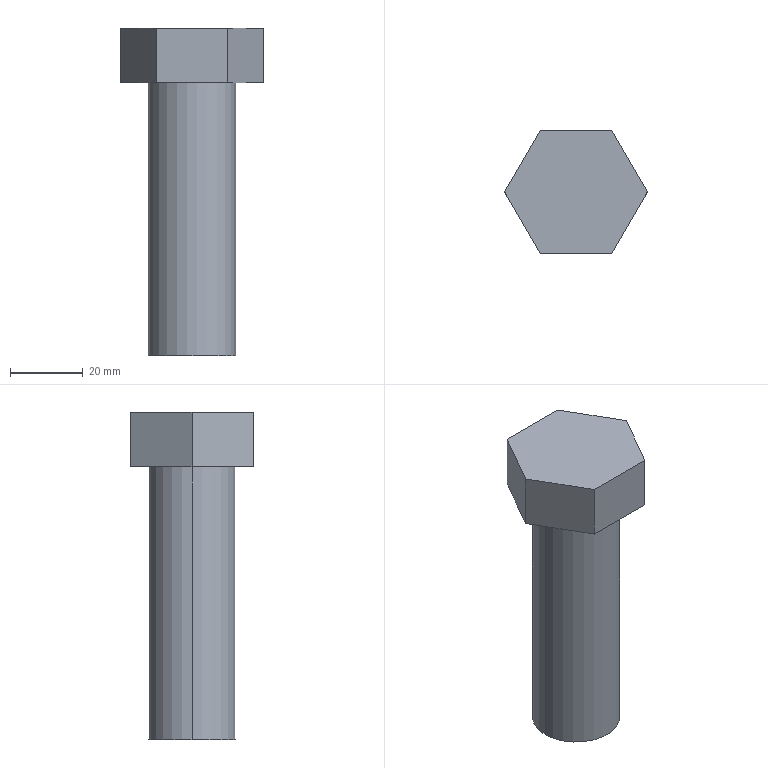Part | STEP file | PN_0027 Punch screw rod | 1 solid | 11 faces | box 39.26 x 34 x 90 mm | volume 48946 mm3 | plane 9 | cylinder 2 | commonest cylinder face diameters 24 x2
STEP:
#1=CARTESIAN_POINT('',(0.,0.,0.));
#2=DIRECTION('',(0.,0.,1.));
#3=DIRECTION('',(1.,0.,0.));
#4=AXIS2_PLACEMENT_3D('',#1,#2,#3);
#5=CARTESIAN_POINT('',(-12.,0.,75.));
#6=VERTEX_POINT('',#5);
#7=CARTESIAN_POINT('',(12.,0.,75.));
#8=VERTEX_POINT('',#7);
#9=CARTESIAN_POINT('',(0.,0.,75.));
#10=DIRECTION('',(0.,0.,-1.));
#11=DIRECTION('',(-1.,0.,0.));
#12=AXIS2_PLACEMENT_3D('',#9,#10,#11);
#13=CIRCLE('',#12,12.);
#14=CARTESIAN_POINT('',(0.,0.,75.));
#15=DIRECTION('',(0.,0.,-1.));
#16=DIRECTION('',(-1.,0.,0.));
#17=AXIS2_PLACEMENT_3D('',#14,#15,#16);
#18=CYLINDRICAL_SURFACE('',#17,12.);
#19=CARTESIAN_POINT('',(0.,0.));
#20=DIRECTION('',(1.,0.));
#21=VECTOR('',#20,1.);
#22=LINE('',#19,#21);
#23=(GEOMETRIC_REPRESENTATION_CONTEXT(2)PARAMETRIC_REPRESENTATION_CONTEXT()REPRESENTATION_CONTEXT('',''));
#24=DEFINITIONAL_REPRESENTATION('',(#22),#23);
#25=PCURVE('',#18,#24);
#26=CARTESIAN_POINT('',(0.,0.,75.));
#27=DIRECTION('',(0.,0.,1.));
#28=DIRECTION('',(1.,0.,0.));
#29=AXIS2_PLACEMENT_3D('',#26,#27,#28);
#30=PLANE('',#29);
#31=CARTESIAN_POINT('',(-12.,0.));
#32=CARTESIAN_POINT('',(-12.,20.785));
#33=CARTESIAN_POINT('',(6.,10.392));
#34=CARTESIAN_POINT('',(24.,0.));
#35=CARTESIAN_POINT('',(6.,-10.392));
#36=CARTESIAN_POINT('',(-12.,-20.785));
#37=CARTESIAN_POINT('',(-12.,0.));
#38=(BOUNDED_CURVE()B_SPLINE_CURVE(2,(#31,#32,#33,#34,#35,#36,#37),.UNSPECIFIED.,.T.,.F.)B_SPLINE_CURVE_WITH_KNOTS((1,2,2,2,2,1),(-2.094,0.,2.094,4.189,6.283,8.378),.UNSPECIFIED.)CURVE()GEOMETRIC_REPRESENTATION_ITEM()RATIONAL_B_SPLINE_CURVE((1.,0.5,1.,0.5,1.,0.5,1.))REPRESENTATION_ITEM(''));
#39=(GEOMETRIC_REPRESENTATION_CONTEXT(2)PARAMETRIC_REPRESENTATION_CONTEXT()REPRESENTATION_CONTEXT('',''));
#40=DEFINITIONAL_REPRESENTATION('',(#38),#39);
#41=PCURVE('',#30,#40);
#42=SURFACE_CURVE('',#13,(#25,#41),.PCURVE_S1.);
#43=EDGE_CURVE('',#6,#8,#42,.T.);
#44=ORIENTED_EDGE('',*,*,#43,.T.);
#45=CARTESIAN_POINT('',(12.,0.,0.));
#46=VERTEX_POINT('',#45);
#47=CARTESIAN_POINT('',(12.,0.,75.));
#48=DIRECTION('',(0.,0.,-1.));
#49=VECTOR('',#48,1.);
#50=LINE('',#47,#49);
#51=CARTESIAN_POINT('',(3.142,0.));
#52=DIRECTION('',(0.,1.));
#53=VECTOR('',#52,1.);
#54=LINE('',#51,#53);
#55=(GEOMETRIC_REPRESENTATION_CONTEXT(2)PARAMETRIC_REPRESENTATION_CONTEXT()REPRESENTATION_CONTEXT('',''));
#56=DEFINITIONAL_REPRESENTATION('',(#54),#55);
#57=PCURVE('',#18,#56);
#58=CARTESIAN_POINT('',(0.,0.,75.));
#59=DIRECTION('',(0.,0.,-1.));
#60=DIRECTION('',(-1.,0.,0.));
#61=AXIS2_PLACEMENT_3D('',#58,#59,#60);
#62=CYLINDRICAL_SURFACE('',#61,12.);
#63=CARTESIAN_POINT('',(3.142,0.));
#64=DIRECTION('',(0.,1.));
#65=VECTOR('',#64,1.);
#66=LINE('',#63,#65);
#67=(GEOMETRIC_REPRESENTATION_CONTEXT(2)PARAMETRIC_REPRESENTATION_CONTEXT()REPRESENTATION_CONTEXT('',''));
#68=DEFINITIONAL_REPRESENTATION('',(#66),#67);
#69=PCURVE('',#62,#68);
#70=SURFACE_CURVE('',#50,(#57,#69),.PCURVE_S1.);
#71=EDGE_CURVE('',#8,#46,#70,.T.);
#72=ORIENTED_EDGE('',*,*,#71,.T.);
#73=CARTESIAN_POINT('',(-12.,0.,0.));
#74=VERTEX_POINT('',#73);
#75=CARTESIAN_POINT('',(0.,0.,0.));
#76=DIRECTION('',(0.,0.,1.));
#77=DIRECTION('',(-1.,0.,0.));
#78=AXIS2_PLACEMENT_3D('',#75,#76,#77);
#79=CIRCLE('',#78,12.);
#80=CARTESIAN_POINT('',(6.283,75.));
#81=DIRECTION('',(-1.,0.));
#82=VECTOR('',#81,1.);
#83=LINE('',#80,#82);
#84=(GEOMETRIC_REPRESENTATION_CONTEXT(2)PARAMETRIC_REPRESENTATION_CONTEXT()REPRESENTATION_CONTEXT('',''));
#85=DEFINITIONAL_REPRESENTATION('',(#83),#84);
#86=PCURVE('',#18,#85);
#87=CARTESIAN_POINT('',(0.,0.,0.));
#88=DIRECTION('',(0.,0.,1.));
#89=DIRECTION('',(1.,0.,0.));
#90=AXIS2_PLACEMENT_3D('',#87,#88,#89);
#91=PLANE('',#90);
#92=CARTESIAN_POINT('',(0.,0.));
#93=DIRECTION('',(-1.,0.));
#94=AXIS2_PLACEMENT_2D('',#92,#93);
#95=CIRCLE('',#94,12.);
#96=(GEOMETRIC_REPRESENTATION_CONTEXT(2)PARAMETRIC_REPRESENTATION_CONTEXT()REPRESENTATION_CONTEXT('',''));
#97=DEFINITIONAL_REPRESENTATION('',(#95),#96);
#98=PCURVE('',#91,#97);
#99=SURFACE_CURVE('',#79,(#86,#98),.PCURVE_S1.);
#100=EDGE_CURVE('',#46,#74,#99,.T.);
#101=ORIENTED_EDGE('',*,*,#100,.T.);
#102=CARTESIAN_POINT('',(-12.,0.,75.));
#103=DIRECTION('',(0.,0.,-1.));
#104=VECTOR('',#103,1.);
#105=LINE('',#102,#104);
#106=CARTESIAN_POINT('',(0.,0.));
#107=DIRECTION('',(0.,1.));
#108=VECTOR('',#107,1.);
#109=LINE('',#106,#108);
#110=(GEOMETRIC_REPRESENTATION_CONTEXT(2)PARAMETRIC_REPRESENTATION_CONTEXT()REPRESENTATION_CONTEXT('',''));
#111=DEFINITIONAL_REPRESENTATION('',(#109),#110);
#112=PCURVE('',#18,#111);
#113=CARTESIAN_POINT('',(6.283,0.));
#114=DIRECTION('',(0.,1.));
#115=VECTOR('',#114,1.);
#116=LINE('',#113,#115);
#117=(GEOMETRIC_REPRESENTATION_CONTEXT(2)PARAMETRIC_REPRESENTATION_CONTEXT()REPRESENTATION_CONTEXT('',''));
#118=DEFINITIONAL_REPRESENTATION('',(#116),#117);
#119=PCURVE('',#62,#118);
#120=SURFACE_CURVE('',#105,(#112,#119),.PCURVE_S1.);
#121=EDGE_CURVE('',#6,#74,#120,.T.);
#122=ORIENTED_EDGE('',*,*,#121,.F.);
#123=EDGE_LOOP('',(#44,#72,#101,#122));
#124=FACE_BOUND('',#123,.T.);
#125=ADVANCED_FACE('',(#124),#18,.T.);
#126=ORIENTED_EDGE('',*,*,#71,.F.);
#127=CARTESIAN_POINT('',(0.,0.,75.));
#128=DIRECTION('',(0.,0.,-1.));
#129=DIRECTION('',(-1.,0.,0.));
#130=AXIS2_PLACEMENT_3D('',#127,#128,#129);
#131=CIRCLE('',#130,12.);
#132=CARTESIAN_POINT('',(0.,0.));
#133=DIRECTION('',(1.,0.));
#134=VECTOR('',#133,1.);
#135=LINE('',#132,#134);
#136=(GEOMETRIC_REPRESENTATION_CONTEXT(2)PARAMETRIC_REPRESENTATION_CONTEXT()REPRESENTATION_CONTEXT('',''));
#137=DEFINITIONAL_REPRESENTATION('',(#135),#136);
#138=PCURVE('',#62,#137);
#139=CARTESIAN_POINT('',(-12.,0.));
#140=CARTESIAN_POINT('',(-12.,20.785));
#141=CARTESIAN_POINT('',(6.,10.392));
#142=CARTESIAN_POINT('',(24.,0.));
#143=CARTESIAN_POINT('',(6.,-10.392));
#144=CARTESIAN_POINT('',(-12.,-20.785));
#145=CARTESIAN_POINT('',(-12.,0.));
#146=(BOUNDED_CURVE()B_SPLINE_CURVE(2,(#139,#140,#141,#142,#143,#144,#145),.UNSPECIFIED.,.T.,.F.)B_SPLINE_CURVE_WITH_KNOTS((1,2,2,2,2,1),(-2.094,0.,2.094,4.189,6.283,8.378),.UNSPECIFIED.)CURVE()GEOMETRIC_REPRESENTATION_ITEM()RATIONAL_B_SPLINE_CURVE((1.,0.5,1.,0.5,1.,0.5,1.))REPRESENTATION_ITEM(''));
#147=(GEOMETRIC_REPRESENTATION_CONTEXT(2)PARAMETRIC_REPRESENTATION_CONTEXT()REPRESENTATION_CONTEXT('',''));
#148=DEFINITIONAL_REPRESENTATION('',(#146),#147);
#149=PCURVE('',#30,#148);
#150=SURFACE_CURVE('',#131,(#138,#149),.PCURVE_S1.);
#151=EDGE_CURVE('',#8,#6,#150,.T.);
#152=ORIENTED_EDGE('',*,*,#151,.T.);
#153=ORIENTED_EDGE('',*,*,#121,.T.);
#154=CARTESIAN_POINT('',(0.,0.,0.));
#155=DIRECTION('',(0.,0.,1.));
#156=DIRECTION('',(-1.,0.,0.));
#157=AXIS2_PLACEMENT_3D('',#154,#155,#156);
#158=CIRCLE('',#157,12.);
#159=CARTESIAN_POINT('',(6.283,75.));
#160=DIRECTION('',(-1.,0.));
#161=VECTOR('',#160,1.);
#162=LINE('',#159,#161);
#163=(GEOMETRIC_REPRESENTATION_CONTEXT(2)PARAMETRIC_REPRESENTATION_CONTEXT()REPRESENTATION_CONTEXT('',''));
#164=DEFINITIONAL_REPRESENTATION('',(#162),#163);
#165=PCURVE('',#62,#164);
#166=CARTESIAN_POINT('',(0.,0.));
#167=DIRECTION('',(-1.,0.));
#168=AXIS2_PLACEMENT_2D('',#166,#167);
#169=CIRCLE('',#168,12.);
#170=(GEOMETRIC_REPRESENTATION_CONTEXT(2)PARAMETRIC_REPRESENTATION_CONTEXT()REPRESENTATION_CONTEXT('',''));
#171=DEFINITIONAL_REPRESENTATION('',(#169),#170);
#172=PCURVE('',#91,#171);
#173=SURFACE_CURVE('',#158,(#165,#172),.PCURVE_S1.);
#174=EDGE_CURVE('',#74,#46,#173,.T.);
#175=ORIENTED_EDGE('',*,*,#174,.T.);
#176=EDGE_LOOP('',(#126,#152,#153,#175));
#177=FACE_BOUND('',#176,.T.);
#178=ADVANCED_FACE('',(#177),#62,.T.);
#179=ORIENTED_EDGE('',*,*,#174,.F.);
#180=ORIENTED_EDGE('',*,*,#100,.F.);
#181=EDGE_LOOP('',(#179,#180));
#182=FACE_BOUND('',#181,.T.);
#183=ADVANCED_FACE('',(#182),#91,.F.);
#184=ORIENTED_EDGE('',*,*,#43,.F.);
#185=ORIENTED_EDGE('',*,*,#151,.F.);
#186=EDGE_LOOP('',(#184,#185));
#187=FACE_BOUND('',#186,.T.);
#188=CARTESIAN_POINT('',(-9.815,-17.,75.));
#189=VERTEX_POINT('',#188);
#190=CARTESIAN_POINT('',(9.815,-17.,75.));
#191=VERTEX_POINT('',#190);
#192=CARTESIAN_POINT('',(0.,-17.,75.));
#193=DIRECTION('',(1.,0.,0.));
#194=VECTOR('',#193,1.);
#195=LINE('',#192,#194);
#196=CARTESIAN_POINT('',(0.,-17.));
#197=DIRECTION('',(1.,0.));
#198=VECTOR('',#197,1.);
#199=LINE('',#196,#198);
#200=(GEOMETRIC_REPRESENTATION_CONTEXT(2)PARAMETRIC_REPRESENTATION_CONTEXT()REPRESENTATION_CONTEXT('',''));
#201=DEFINITIONAL_REPRESENTATION('',(#199),#200);
#202=PCURVE('',#30,#201);
#203=CARTESIAN_POINT('',(-9.815,-17.,90.));
#204=DIRECTION('',(0.,1.,0.));
#205=DIRECTION('',(-1.,0.,0.));
#206=AXIS2_PLACEMENT_3D('',#203,#204,#205);
#207=PLANE('',#206);
#208=CARTESIAN_POINT('',(-9.815,-15.));
#209=DIRECTION('',(-1.,0.));
#210=VECTOR('',#209,1.);
#211=LINE('',#208,#210);
#212=(GEOMETRIC_REPRESENTATION_CONTEXT(2)PARAMETRIC_REPRESENTATION_CONTEXT()REPRESENTATION_CONTEXT('',''));
#213=DEFINITIONAL_REPRESENTATION('',(#211),#212);
#214=PCURVE('',#207,#213);
#215=SURFACE_CURVE('',#195,(#202,#214),.PCURVE_S1.);
#216=EDGE_CURVE('',#189,#191,#215,.T.);
#217=ORIENTED_EDGE('',*,*,#216,.F.);
#218=CARTESIAN_POINT('',(-19.63,0.,75.));
#219=VERTEX_POINT('',#218);
#220=CARTESIAN_POINT('',(-19.63,0.,75.));
#221=DIRECTION('',(0.5,-0.866,0.));
#222=VECTOR('',#221,1.);
#223=LINE('',#220,#222);
#224=CARTESIAN_POINT('',(-19.63,0.));
#225=DIRECTION('',(0.5,-0.866));
#226=VECTOR('',#225,1.);
#227=LINE('',#224,#226);
#228=(GEOMETRIC_REPRESENTATION_CONTEXT(2)PARAMETRIC_REPRESENTATION_CONTEXT()REPRESENTATION_CONTEXT('',''));
#229=DEFINITIONAL_REPRESENTATION('',(#227),#228);
#230=PCURVE('',#30,#229);
#231=CARTESIAN_POINT('',(-19.63,0.,90.));
#232=DIRECTION('',(0.866,0.5,0.));
#233=DIRECTION('',(-0.5,0.866,0.));
#234=AXIS2_PLACEMENT_3D('',#231,#232,#233);
#235=PLANE('',#234);
#236=CARTESIAN_POINT('',(0.,-15.));
#237=DIRECTION('',(-1.,0.));
#238=VECTOR('',#237,1.);
#239=LINE('',#236,#238);
#240=(GEOMETRIC_REPRESENTATION_CONTEXT(2)PARAMETRIC_REPRESENTATION_CONTEXT()REPRESENTATION_CONTEXT('',''));
#241=DEFINITIONAL_REPRESENTATION('',(#239),#240);
#242=PCURVE('',#235,#241);
#243=SURFACE_CURVE('',#223,(#230,#242),.PCURVE_S1.);
#244=EDGE_CURVE('',#219,#189,#243,.T.);
#245=ORIENTED_EDGE('',*,*,#244,.F.);
#246=CARTESIAN_POINT('',(-9.815,17.,75.));
#247=VERTEX_POINT('',#246);
#248=CARTESIAN_POINT('',(-9.815,17.,75.));
#249=DIRECTION('',(-0.5,-0.866,0.));
#250=VECTOR('',#249,1.);
#251=LINE('',#248,#250);
#252=CARTESIAN_POINT('',(-9.815,17.));
#253=DIRECTION('',(-0.5,-0.866));
#254=VECTOR('',#253,1.);
#255=LINE('',#252,#254);
#256=(GEOMETRIC_REPRESENTATION_CONTEXT(2)PARAMETRIC_REPRESENTATION_CONTEXT()REPRESENTATION_CONTEXT('',''));
#257=DEFINITIONAL_REPRESENTATION('',(#255),#256);
#258=PCURVE('',#30,#257);
#259=CARTESIAN_POINT('',(-9.815,17.,90.));
#260=DIRECTION('',(0.866,-0.5,0.));
#261=DIRECTION('',(0.5,0.866,0.));
#262=AXIS2_PLACEMENT_3D('',#259,#260,#261);
#263=PLANE('',#262);
#264=CARTESIAN_POINT('',(0.,-15.));
#265=DIRECTION('',(-1.,0.));
#266=VECTOR('',#265,1.);
#267=LINE('',#264,#266);
#268=(GEOMETRIC_REPRESENTATION_CONTEXT(2)PARAMETRIC_REPRESENTATION_CONTEXT()REPRESENTATION_CONTEXT('',''));
#269=DEFINITIONAL_REPRESENTATION('',(#267),#268);
#270=PCURVE('',#263,#269);
#271=SURFACE_CURVE('',#251,(#258,#270),.PCURVE_S1.);
#272=EDGE_CURVE('',#247,#219,#271,.T.);
#273=ORIENTED_EDGE('',*,*,#272,.F.);
#274=CARTESIAN_POINT('',(9.815,17.,75.));
#275=VERTEX_POINT('',#274);
#276=CARTESIAN_POINT('',(0.,17.,75.));
#277=DIRECTION('',(-1.,0.,0.));
#278=VECTOR('',#277,1.);
#279=LINE('',#276,#278);
#280=CARTESIAN_POINT('',(0.,17.));
#281=DIRECTION('',(-1.,0.));
#282=VECTOR('',#281,1.);
#283=LINE('',#280,#282);
#284=(GEOMETRIC_REPRESENTATION_CONTEXT(2)PARAMETRIC_REPRESENTATION_CONTEXT()REPRESENTATION_CONTEXT('',''));
#285=DEFINITIONAL_REPRESENTATION('',(#283),#284);
#286=PCURVE('',#30,#285);
#287=CARTESIAN_POINT('',(9.815,17.,90.));
#288=DIRECTION('',(0.,-1.,0.));
#289=DIRECTION('',(1.,0.,0.));
#290=AXIS2_PLACEMENT_3D('',#287,#288,#289);
#291=PLANE('',#290);
#292=CARTESIAN_POINT('',(-9.815,-15.));
#293=DIRECTION('',(-1.,0.));
#294=VECTOR('',#293,1.);
#295=LINE('',#292,#294);
#296=(GEOMETRIC_REPRESENTATION_CONTEXT(2)PARAMETRIC_REPRESENTATION_CONTEXT()REPRESENTATION_CONTEXT('',''));
#297=DEFINITIONAL_REPRESENTATION('',(#295),#296);
#298=PCURVE('',#291,#297);
#299=SURFACE_CURVE('',#279,(#286,#298),.PCURVE_S1.);
#300=EDGE_CURVE('',#275,#247,#299,.T.);
#301=ORIENTED_EDGE('',*,*,#300,.F.);
#302=CARTESIAN_POINT('',(19.63,0.,75.));
#303=VERTEX_POINT('',#302);
#304=CARTESIAN_POINT('',(19.63,0.,75.));
#305=DIRECTION('',(-0.5,0.866,0.));
#306=VECTOR('',#305,1.);
#307=LINE('',#304,#306);
#308=CARTESIAN_POINT('',(19.63,0.));
#309=DIRECTION('',(-0.5,0.866));
#310=VECTOR('',#309,1.);
#311=LINE('',#308,#310);
#312=(GEOMETRIC_REPRESENTATION_CONTEXT(2)PARAMETRIC_REPRESENTATION_CONTEXT()REPRESENTATION_CONTEXT('',''));
#313=DEFINITIONAL_REPRESENTATION('',(#311),#312);
#314=PCURVE('',#30,#313);
#315=CARTESIAN_POINT('',(19.63,0.,90.));
#316=DIRECTION('',(-0.866,-0.5,0.));
#317=DIRECTION('',(0.5,-0.866,0.));
#318=AXIS2_PLACEMENT_3D('',#315,#316,#317);
#319=PLANE('',#318);
#320=CARTESIAN_POINT('',(0.,-15.));
#321=DIRECTION('',(-1.,0.));
#322=VECTOR('',#321,1.);
#323=LINE('',#320,#322);
#324=(GEOMETRIC_REPRESENTATION_CONTEXT(2)PARAMETRIC_REPRESENTATION_CONTEXT()REPRESENTATION_CONTEXT('',''));
#325=DEFINITIONAL_REPRESENTATION('',(#323),#324);
#326=PCURVE('',#319,#325);
#327=SURFACE_CURVE('',#307,(#314,#326),.PCURVE_S1.);
#328=EDGE_CURVE('',#303,#275,#327,.T.);
#329=ORIENTED_EDGE('',*,*,#328,.F.);
#330=CARTESIAN_POINT('',(9.815,-17.,75.));
#331=DIRECTION('',(0.5,0.866,0.));
#332=VECTOR('',#331,1.);
#333=LINE('',#330,#332);
#334=CARTESIAN_POINT('',(9.815,-17.));
#335=DIRECTION('',(0.5,0.866));
#336=VECTOR('',#335,1.);
#337=LINE('',#334,#336);
#338=(GEOMETRIC_REPRESENTATION_CONTEXT(2)PARAMETRIC_REPRESENTATION_CONTEXT()REPRESENTATION_CONTEXT('',''));
#339=DEFINITIONAL_REPRESENTATION('',(#337),#338);
#340=PCURVE('',#30,#339);
#341=CARTESIAN_POINT('',(9.815,-17.,90.));
#342=DIRECTION('',(-0.866,0.5,0.));
#343=DIRECTION('',(-0.5,-0.866,0.));
#344=AXIS2_PLACEMENT_3D('',#341,#342,#343);
#345=PLANE('',#344);
#346=CARTESIAN_POINT('',(0.,-15.));
#347=DIRECTION('',(-1.,0.));
#348=VECTOR('',#347,1.);
#349=LINE('',#346,#348);
#350=(GEOMETRIC_REPRESENTATION_CONTEXT(2)PARAMETRIC_REPRESENTATION_CONTEXT()REPRESENTATION_CONTEXT('',''));
#351=DEFINITIONAL_REPRESENTATION('',(#349),#350);
#352=PCURVE('',#345,#351);
#353=SURFACE_CURVE('',#333,(#340,#352),.PCURVE_S1.);
#354=EDGE_CURVE('',#191,#303,#353,.T.);
#355=ORIENTED_EDGE('',*,*,#354,.F.);
#356=EDGE_LOOP('',(#217,#245,#273,#301,#329,#355));
#357=FACE_BOUND('',#356,.T.);
#358=ADVANCED_FACE('',(#187,#357),#30,.F.);
#359=CARTESIAN_POINT('',(19.63,0.,90.));
#360=VERTEX_POINT('',#359);
#361=CARTESIAN_POINT('',(19.63,0.,90.));
#362=DIRECTION('',(0.,0.,-1.));
#363=VECTOR('',#362,1.);
#364=LINE('',#361,#363);
#365=CARTESIAN_POINT('',(-19.63,0.));
#366=DIRECTION('',(0.,-1.));
#367=VECTOR('',#366,1.);
#368=LINE('',#365,#367);
#369=(GEOMETRIC_REPRESENTATION_CONTEXT(2)PARAMETRIC_REPRESENTATION_CONTEXT()REPRESENTATION_CONTEXT('',''));
#370=DEFINITIONAL_REPRESENTATION('',(#368),#369);
#371=PCURVE('',#345,#370);
#372=CARTESIAN_POINT('',(0.,0.));
#373=DIRECTION('',(0.,-1.));
#374=VECTOR('',#373,1.);
#375=LINE('',#372,#374);
#376=(GEOMETRIC_REPRESENTATION_CONTEXT(2)PARAMETRIC_REPRESENTATION_CONTEXT()REPRESENTATION_CONTEXT('',''));
#377=DEFINITIONAL_REPRESENTATION('',(#375),#376);
#378=PCURVE('',#319,#377);
#379=SURFACE_CURVE('',#364,(#371,#378),.PCURVE_S1.);
#380=EDGE_CURVE('',#360,#303,#379,.T.);
#381=ORIENTED_EDGE('',*,*,#380,.F.);
#382=CARTESIAN_POINT('',(9.815,-17.,90.));
#383=VERTEX_POINT('',#382);
#384=CARTESIAN_POINT('',(9.815,-17.,90.));
#385=DIRECTION('',(0.5,0.866,0.));
#386=VECTOR('',#385,1.);
#387=LINE('',#384,#386);
#388=CARTESIAN_POINT('',(0.,0.));
#389=DIRECTION('',(-1.,0.));
#390=VECTOR('',#389,1.);
#391=LINE('',#388,#390);
#392=(GEOMETRIC_REPRESENTATION_CONTEXT(2)PARAMETRIC_REPRESENTATION_CONTEXT()REPRESENTATION_CONTEXT('',''));
#393=DEFINITIONAL_REPRESENTATION('',(#391),#392);
#394=PCURVE('',#345,#393);
#395=CARTESIAN_POINT('',(0.,0.,90.));
#396=DIRECTION('',(0.,0.,1.));
#397=DIRECTION('',(1.,0.,0.));
#398=AXIS2_PLACEMENT_3D('',#395,#396,#397);
#399=PLANE('',#398);
#400=CARTESIAN_POINT('',(9.815,-17.));
#401=DIRECTION('',(0.5,0.866));
#402=VECTOR('',#401,1.);
#403=LINE('',#400,#402);
#404=(GEOMETRIC_REPRESENTATION_CONTEXT(2)PARAMETRIC_REPRESENTATION_CONTEXT()REPRESENTATION_CONTEXT('',''));
#405=DEFINITIONAL_REPRESENTATION('',(#403),#404);
#406=PCURVE('',#399,#405);
#407=SURFACE_CURVE('',#387,(#394,#406),.PCURVE_S1.);
#408=EDGE_CURVE('',#383,#360,#407,.T.);
#409=ORIENTED_EDGE('',*,*,#408,.F.);
#410=CARTESIAN_POINT('',(9.815,-17.,90.));
#411=DIRECTION('',(0.,0.,1.));
#412=VECTOR('',#411,1.);
#413=LINE('',#410,#412);
#414=CARTESIAN_POINT('',(0.,0.));
#415=DIRECTION('',(0.,1.));
#416=VECTOR('',#415,1.);
#417=LINE('',#414,#416);
#418=(GEOMETRIC_REPRESENTATION_CONTEXT(2)PARAMETRIC_REPRESENTATION_CONTEXT()REPRESENTATION_CONTEXT('',''));
#419=DEFINITIONAL_REPRESENTATION('',(#417),#418);
#420=PCURVE('',#345,#419);
#421=CARTESIAN_POINT('',(-19.63,0.));
#422=DIRECTION('',(0.,1.));
#423=VECTOR('',#422,1.);
#424=LINE('',#421,#423);
#425=(GEOMETRIC_REPRESENTATION_CONTEXT(2)PARAMETRIC_REPRESENTATION_CONTEXT()REPRESENTATION_CONTEXT('',''));
#426=DEFINITIONAL_REPRESENTATION('',(#424),#425);
#427=PCURVE('',#207,#426);
#428=SURFACE_CURVE('',#413,(#420,#427),.PCURVE_S1.);
#429=EDGE_CURVE('',#191,#383,#428,.T.);
#430=ORIENTED_EDGE('',*,*,#429,.F.);
#431=ORIENTED_EDGE('',*,*,#354,.T.);
#432=EDGE_LOOP('',(#381,#409,#430,#431));
#433=FACE_BOUND('',#432,.T.);
#434=ADVANCED_FACE('',(#433),#345,.F.);
#435=ORIENTED_EDGE('',*,*,#429,.T.);
#436=CARTESIAN_POINT('',(-9.815,-17.,90.));
#437=VERTEX_POINT('',#436);
#438=CARTESIAN_POINT('',(-9.815,-17.,90.));
#439=DIRECTION('',(1.,0.,0.));
#440=VECTOR('',#439,1.);
#441=LINE('',#438,#440);
#442=CARTESIAN_POINT('',(0.,0.));
#443=DIRECTION('',(-1.,0.));
#444=VECTOR('',#443,1.);
#445=LINE('',#442,#444);
#446=(GEOMETRIC_REPRESENTATION_CONTEXT(2)PARAMETRIC_REPRESENTATION_CONTEXT()REPRESENTATION_CONTEXT('',''));
#447=DEFINITIONAL_REPRESENTATION('',(#445),#446);
#448=PCURVE('',#207,#447);
#449=CARTESIAN_POINT('',(-9.815,-17.));
#450=DIRECTION('',(1.,0.));
#451=VECTOR('',#450,1.);
#452=LINE('',#449,#451);
#453=(GEOMETRIC_REPRESENTATION_CONTEXT(2)PARAMETRIC_REPRESENTATION_CONTEXT()REPRESENTATION_CONTEXT('',''));
#454=DEFINITIONAL_REPRESENTATION('',(#452),#453);
#455=PCURVE('',#399,#454);
#456=SURFACE_CURVE('',#441,(#448,#455),.PCURVE_S1.);
#457=EDGE_CURVE('',#437,#383,#456,.T.);
#458=ORIENTED_EDGE('',*,*,#457,.F.);
#459=CARTESIAN_POINT('',(-9.815,-17.,90.));
#460=DIRECTION('',(0.,0.,1.));
#461=VECTOR('',#460,1.);
#462=LINE('',#459,#461);
#463=CARTESIAN_POINT('',(0.,0.));
#464=DIRECTION('',(0.,1.));
#465=VECTOR('',#464,1.);
#466=LINE('',#463,#465);
#467=(GEOMETRIC_REPRESENTATION_CONTEXT(2)PARAMETRIC_REPRESENTATION_CONTEXT()REPRESENTATION_CONTEXT('',''));
#468=DEFINITIONAL_REPRESENTATION('',(#466),#467);
#469=PCURVE('',#207,#468);
#470=CARTESIAN_POINT('',(-19.63,0.));
#471=DIRECTION('',(0.,1.));
#472=VECTOR('',#471,1.);
#473=LINE('',#470,#472);
#474=(GEOMETRIC_REPRESENTATION_CONTEXT(2)PARAMETRIC_REPRESENTATION_CONTEXT()REPRESENTATION_CONTEXT('',''));
#475=DEFINITIONAL_REPRESENTATION('',(#473),#474);
#476=PCURVE('',#235,#475);
#477=SURFACE_CURVE('',#462,(#469,#476),.PCURVE_S1.);
#478=EDGE_CURVE('',#189,#437,#477,.T.);
#479=ORIENTED_EDGE('',*,*,#478,.F.);
#480=ORIENTED_EDGE('',*,*,#216,.T.);
#481=EDGE_LOOP('',(#435,#458,#479,#480));
#482=FACE_BOUND('',#481,.T.);
#483=ADVANCED_FACE('',(#482),#207,.F.);
#484=ORIENTED_EDGE('',*,*,#478,.T.);
#485=CARTESIAN_POINT('',(-19.63,0.,90.));
#486=VERTEX_POINT('',#485);
#487=CARTESIAN_POINT('',(-19.63,0.,90.));
#488=DIRECTION('',(0.5,-0.866,0.));
#489=VECTOR('',#488,1.);
#490=LINE('',#487,#489);
#491=CARTESIAN_POINT('',(0.,0.));
#492=DIRECTION('',(-1.,0.));
#493=VECTOR('',#492,1.);
#494=LINE('',#491,#493);
#495=(GEOMETRIC_REPRESENTATION_CONTEXT(2)PARAMETRIC_REPRESENTATION_CONTEXT()REPRESENTATION_CONTEXT('',''));
#496=DEFINITIONAL_REPRESENTATION('',(#494),#495);
#497=PCURVE('',#235,#496);
#498=CARTESIAN_POINT('',(-19.63,0.));
#499=DIRECTION('',(0.5,-0.866));
#500=VECTOR('',#499,1.);
#501=LINE('',#498,#500);
#502=(GEOMETRIC_REPRESENTATION_CONTEXT(2)PARAMETRIC_REPRESENTATION_CONTEXT()REPRESENTATION_CONTEXT('',''));
#503=DEFINITIONAL_REPRESENTATION('',(#501),#502);
#504=PCURVE('',#399,#503);
#505=SURFACE_CURVE('',#490,(#497,#504),.PCURVE_S1.);
#506=EDGE_CURVE('',#486,#437,#505,.T.);
#507=ORIENTED_EDGE('',*,*,#506,.F.);
#508=CARTESIAN_POINT('',(-19.63,0.,90.));
#509=DIRECTION('',(0.,0.,1.));
#510=VECTOR('',#509,1.);
#511=LINE('',#508,#510);
#512=CARTESIAN_POINT('',(0.,0.));
#513=DIRECTION('',(0.,1.));
#514=VECTOR('',#513,1.);
#515=LINE('',#512,#514);
#516=(GEOMETRIC_REPRESENTATION_CONTEXT(2)PARAMETRIC_REPRESENTATION_CONTEXT()REPRESENTATION_CONTEXT('',''));
#517=DEFINITIONAL_REPRESENTATION('',(#515),#516);
#518=PCURVE('',#235,#517);
#519=CARTESIAN_POINT('',(-19.63,0.));
#520=DIRECTION('',(0.,1.));
#521=VECTOR('',#520,1.);
#522=LINE('',#519,#521);
#523=(GEOMETRIC_REPRESENTATION_CONTEXT(2)PARAMETRIC_REPRESENTATION_CONTEXT()REPRESENTATION_CONTEXT('',''));
#524=DEFINITIONAL_REPRESENTATION('',(#522),#523);
#525=PCURVE('',#263,#524);
#526=SURFACE_CURVE('',#511,(#518,#525),.PCURVE_S1.);
#527=EDGE_CURVE('',#219,#486,#526,.T.);
#528=ORIENTED_EDGE('',*,*,#527,.F.);
#529=ORIENTED_EDGE('',*,*,#244,.T.);
#530=EDGE_LOOP('',(#484,#507,#528,#529));
#531=FACE_BOUND('',#530,.T.);
#532=ADVANCED_FACE('',(#531),#235,.F.);
#533=ORIENTED_EDGE('',*,*,#527,.T.);
#534=CARTESIAN_POINT('',(-9.815,17.,90.));
#535=VERTEX_POINT('',#534);
#536=CARTESIAN_POINT('',(-9.815,17.,90.));
#537=DIRECTION('',(-0.5,-0.866,0.));
#538=VECTOR('',#537,1.);
#539=LINE('',#536,#538);
#540=CARTESIAN_POINT('',(0.,0.));
#541=DIRECTION('',(-1.,0.));
#542=VECTOR('',#541,1.);
#543=LINE('',#540,#542);
#544=(GEOMETRIC_REPRESENTATION_CONTEXT(2)PARAMETRIC_REPRESENTATION_CONTEXT()REPRESENTATION_CONTEXT('',''));
#545=DEFINITIONAL_REPRESENTATION('',(#543),#544);
#546=PCURVE('',#263,#545);
#547=CARTESIAN_POINT('',(-9.815,17.));
#548=DIRECTION('',(-0.5,-0.866));
#549=VECTOR('',#548,1.);
#550=LINE('',#547,#549);
#551=(GEOMETRIC_REPRESENTATION_CONTEXT(2)PARAMETRIC_REPRESENTATION_CONTEXT()REPRESENTATION_CONTEXT('',''));
#552=DEFINITIONAL_REPRESENTATION('',(#550),#551);
#553=PCURVE('',#399,#552);
#554=SURFACE_CURVE('',#539,(#546,#553),.PCURVE_S1.);
#555=EDGE_CURVE('',#535,#486,#554,.T.);
#556=ORIENTED_EDGE('',*,*,#555,.F.);
#557=CARTESIAN_POINT('',(-9.815,17.,90.));
#558=DIRECTION('',(0.,0.,1.));
#559=VECTOR('',#558,1.);
#560=LINE('',#557,#559);
#561=CARTESIAN_POINT('',(0.,0.));
#562=DIRECTION('',(0.,1.));
#563=VECTOR('',#562,1.);
#564=LINE('',#561,#563);
#565=(GEOMETRIC_REPRESENTATION_CONTEXT(2)PARAMETRIC_REPRESENTATION_CONTEXT()REPRESENTATION_CONTEXT('',''));
#566=DEFINITIONAL_REPRESENTATION('',(#564),#565);
#567=PCURVE('',#263,#566);
#568=CARTESIAN_POINT('',(-19.63,0.));
#569=DIRECTION('',(0.,1.));
#570=VECTOR('',#569,1.);
#571=LINE('',#568,#570);
#572=(GEOMETRIC_REPRESENTATION_CONTEXT(2)PARAMETRIC_REPRESENTATION_CONTEXT()REPRESENTATION_CONTEXT('',''));
#573=DEFINITIONAL_REPRESENTATION('',(#571),#572);
#574=PCURVE('',#291,#573);
#575=SURFACE_CURVE('',#560,(#567,#574),.PCURVE_S1.);
#576=EDGE_CURVE('',#247,#535,#575,.T.);
#577=ORIENTED_EDGE('',*,*,#576,.F.);
#578=ORIENTED_EDGE('',*,*,#272,.T.);
#579=EDGE_LOOP('',(#533,#556,#577,#578));
#580=FACE_BOUND('',#579,.T.);
#581=ADVANCED_FACE('',(#580),#263,.F.);
#582=ORIENTED_EDGE('',*,*,#576,.T.);
#583=CARTESIAN_POINT('',(9.815,17.,90.));
#584=VERTEX_POINT('',#583);
#585=CARTESIAN_POINT('',(9.815,17.,90.));
#586=DIRECTION('',(-1.,0.,0.));
#587=VECTOR('',#586,1.);
#588=LINE('',#585,#587);
#589=CARTESIAN_POINT('',(0.,0.));
#590=DIRECTION('',(-1.,0.));
#591=VECTOR('',#590,1.);
#592=LINE('',#589,#591);
#593=(GEOMETRIC_REPRESENTATION_CONTEXT(2)PARAMETRIC_REPRESENTATION_CONTEXT()REPRESENTATION_CONTEXT('',''));
#594=DEFINITIONAL_REPRESENTATION('',(#592),#593);
#595=PCURVE('',#291,#594);
#596=CARTESIAN_POINT('',(9.815,17.));
#597=DIRECTION('',(-1.,0.));
#598=VECTOR('',#597,1.);
#599=LINE('',#596,#598);
#600=(GEOMETRIC_REPRESENTATION_CONTEXT(2)PARAMETRIC_REPRESENTATION_CONTEXT()REPRESENTATION_CONTEXT('',''));
#601=DEFINITIONAL_REPRESENTATION('',(#599),#600);
#602=PCURVE('',#399,#601);
#603=SURFACE_CURVE('',#588,(#595,#602),.PCURVE_S1.);
#604=EDGE_CURVE('',#584,#535,#603,.T.);
#605=ORIENTED_EDGE('',*,*,#604,.F.);
#606=CARTESIAN_POINT('',(9.815,17.,90.));
#607=DIRECTION('',(0.,0.,1.));
#608=VECTOR('',#607,1.);
#609=LINE('',#606,#608);
#610=CARTESIAN_POINT('',(0.,0.));
#611=DIRECTION('',(0.,1.));
#612=VECTOR('',#611,1.);
#613=LINE('',#610,#612);
#614=(GEOMETRIC_REPRESENTATION_CONTEXT(2)PARAMETRIC_REPRESENTATION_CONTEXT()REPRESENTATION_CONTEXT('',''));
#615=DEFINITIONAL_REPRESENTATION('',(#613),#614);
#616=PCURVE('',#291,#615);
#617=CARTESIAN_POINT('',(-19.63,0.));
#618=DIRECTION('',(0.,1.));
#619=VECTOR('',#618,1.);
#620=LINE('',#617,#619);
#621=(GEOMETRIC_REPRESENTATION_CONTEXT(2)PARAMETRIC_REPRESENTATION_CONTEXT()REPRESENTATION_CONTEXT('',''));
#622=DEFINITIONAL_REPRESENTATION('',(#620),#621);
#623=PCURVE('',#319,#622);
#624=SURFACE_CURVE('',#609,(#616,#623),.PCURVE_S1.);
#625=EDGE_CURVE('',#275,#584,#624,.T.);
#626=ORIENTED_EDGE('',*,*,#625,.F.);
#627=ORIENTED_EDGE('',*,*,#300,.T.);
#628=EDGE_LOOP('',(#582,#605,#626,#627));
#629=FACE_BOUND('',#628,.T.);
#630=ADVANCED_FACE('',(#629),#291,.F.);
#631=ORIENTED_EDGE('',*,*,#625,.T.);
#632=CARTESIAN_POINT('',(19.63,0.,90.));
#633=DIRECTION('',(-0.5,0.866,0.));
#634=VECTOR('',#633,1.);
#635=LINE('',#632,#634);
#636=CARTESIAN_POINT('',(0.,0.));
#637=DIRECTION('',(-1.,0.));
#638=VECTOR('',#637,1.);
#639=LINE('',#636,#638);
#640=(GEOMETRIC_REPRESENTATION_CONTEXT(2)PARAMETRIC_REPRESENTATION_CONTEXT()REPRESENTATION_CONTEXT('',''));
#641=DEFINITIONAL_REPRESENTATION('',(#639),#640);
#642=PCURVE('',#319,#641);
#643=CARTESIAN_POINT('',(19.63,0.));
#644=DIRECTION('',(-0.5,0.866));
#645=VECTOR('',#644,1.);
#646=LINE('',#643,#645);
#647=(GEOMETRIC_REPRESENTATION_CONTEXT(2)PARAMETRIC_REPRESENTATION_CONTEXT()REPRESENTATION_CONTEXT('',''));
#648=DEFINITIONAL_REPRESENTATION('',(#646),#647);
#649=PCURVE('',#399,#648);
#650=SURFACE_CURVE('',#635,(#642,#649),.PCURVE_S1.);
#651=EDGE_CURVE('',#360,#584,#650,.T.);
#652=ORIENTED_EDGE('',*,*,#651,.F.);
#653=ORIENTED_EDGE('',*,*,#380,.T.);
#654=ORIENTED_EDGE('',*,*,#328,.T.);
#655=EDGE_LOOP('',(#631,#652,#653,#654));
#656=FACE_BOUND('',#655,.T.);
#657=ADVANCED_FACE('',(#656),#319,.F.);
#658=ORIENTED_EDGE('',*,*,#506,.T.);
#659=ORIENTED_EDGE('',*,*,#457,.T.);
#660=ORIENTED_EDGE('',*,*,#408,.T.);
#661=ORIENTED_EDGE('',*,*,#651,.T.);
#662=ORIENTED_EDGE('',*,*,#604,.T.);
#663=ORIENTED_EDGE('',*,*,#555,.T.);
#664=EDGE_LOOP('',(#658,#659,#660,#661,#662,#663));
#665=FACE_BOUND('',#664,.T.);
#666=ADVANCED_FACE('',(#665),#399,.T.);
#667=CLOSED_SHELL('',(#125,#178,#183,#358,#434,#483,#532,#581,#630,#657,#666));
#668=MANIFOLD_SOLID_BREP('',#667);
#669=(LENGTH_UNIT()NAMED_UNIT(*)SI_UNIT(.MILLI.,.METRE.));
#670=UNCERTAINTY_MEASURE_WITH_UNIT(LENGTH_MEASURE(0.0000001),#669,'','');
#671=(NAMED_UNIT(*)PLANE_ANGLE_UNIT()SI_UNIT($,.RADIAN.));
#672=(NAMED_UNIT(*)SI_UNIT($,.STERADIAN.)SOLID_ANGLE_UNIT());
#673=(GEOMETRIC_REPRESENTATION_CONTEXT(3)GLOBAL_UNCERTAINTY_ASSIGNED_CONTEXT((#670))GLOBAL_UNIT_ASSIGNED_CONTEXT((#669,#671,#672))REPRESENTATION_CONTEXT('',''));
#674=ADVANCED_BREP_SHAPE_REPRESENTATION('',(#4,#668),#673);